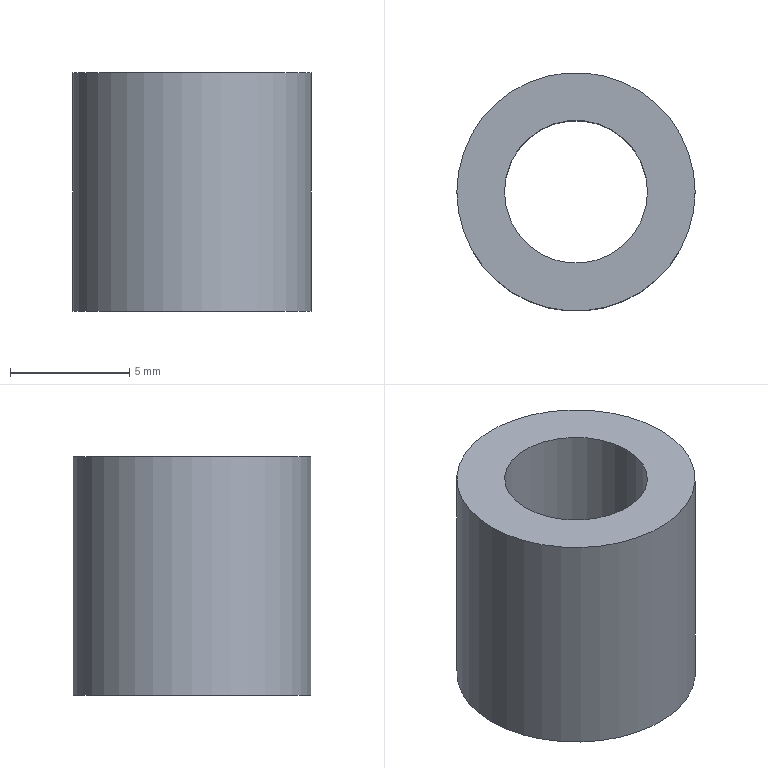Part | NX | features DATUM_CSYS 1, EXTRUDE 1 | 1 solid | 4 faces | box 10 x 10 x 10 mm | volume 502.655 mm3 | cylinder 2 | plane 2 | commonest cylinder face diameters 6 x1 10 x1
STEP:
#1=CARTESIAN_POINT('',(5.,0.,10.));
#2=VERTEX_POINT('',#1);
#3=CARTESIAN_POINT('',(0.,0.,10.));
#4=DIRECTION('',(0.,0.,1.));
#5=DIRECTION('',(1.,0.,0.));
#6=AXIS2_PLACEMENT_3D('',#3,#4,#5);
#7=CIRCLE('',#6,5.);
#8=EDGE_CURVE('',#2,#2,#7,.T.);
#9=ORIENTED_EDGE('',*,*,#8,.F.);
#10=EDGE_LOOP('',(#9));
#11=FACE_BOUND('',#10,.T.);
#12=CARTESIAN_POINT('',(5.,0.,0.));
#13=VERTEX_POINT('',#12);
#14=CARTESIAN_POINT('',(0.,0.,0.));
#15=DIRECTION('',(0.,0.,1.));
#16=DIRECTION('',(1.,0.,0.));
#17=AXIS2_PLACEMENT_3D('',#14,#15,#16);
#18=CIRCLE('',#17,5.);
#19=EDGE_CURVE('',#13,#13,#18,.T.);
#20=ORIENTED_EDGE('',*,*,#19,.T.);
#21=EDGE_LOOP('',(#20));
#22=FACE_BOUND('',#21,.T.);
#23=CARTESIAN_POINT('',(0.,0.,10.));
#24=DIRECTION('',(0.,0.,-1.));
#25=DIRECTION('',(-1.,0.,0.));
#26=AXIS2_PLACEMENT_3D('',#23,#24,#25);
#27=CYLINDRICAL_SURFACE('',#26,5.);
#28=ADVANCED_FACE('',(#11,#22),#27,.T.);
#29=CARTESIAN_POINT('',(3.,0.,10.));
#30=VERTEX_POINT('',#29);
#31=CARTESIAN_POINT('',(0.,0.,10.));
#32=DIRECTION('',(0.,0.,-1.));
#33=DIRECTION('',(1.,0.,0.));
#34=AXIS2_PLACEMENT_3D('',#31,#32,#33);
#35=CIRCLE('',#34,3.);
#36=EDGE_CURVE('',#30,#30,#35,.T.);
#37=ORIENTED_EDGE('',*,*,#36,.F.);
#38=EDGE_LOOP('',(#37));
#39=FACE_BOUND('',#38,.T.);
#40=CARTESIAN_POINT('',(3.,0.,0.));
#41=VERTEX_POINT('',#40);
#42=CARTESIAN_POINT('',(0.,0.,0.));
#43=DIRECTION('',(0.,0.,-1.));
#44=DIRECTION('',(1.,0.,0.));
#45=AXIS2_PLACEMENT_3D('',#42,#43,#44);
#46=CIRCLE('',#45,3.);
#47=EDGE_CURVE('',#41,#41,#46,.T.);
#48=ORIENTED_EDGE('',*,*,#47,.T.);
#49=EDGE_LOOP('',(#48));
#50=FACE_BOUND('',#49,.T.);
#51=CARTESIAN_POINT('',(0.,0.,10.));
#52=DIRECTION('',(0.,0.,-1.));
#53=DIRECTION('',(-1.,0.,0.));
#54=AXIS2_PLACEMENT_3D('',#51,#52,#53);
#55=CYLINDRICAL_SURFACE('',#54,3.);
#56=ADVANCED_FACE('',(#39,#50),#55,.F.);
#57=ORIENTED_EDGE('',*,*,#8,.T.);
#58=EDGE_LOOP('',(#57));
#59=FACE_BOUND('',#58,.T.);
#60=ORIENTED_EDGE('',*,*,#36,.T.);
#61=EDGE_LOOP('',(#60));
#62=FACE_BOUND('',#61,.T.);
#63=CARTESIAN_POINT('',(0.,0.,10.));
#64=DIRECTION('',(0.,0.,1.));
#65=DIRECTION('',(1.,0.,0.));
#66=AXIS2_PLACEMENT_3D('',#63,#64,#65);
#67=PLANE('',#66);
#68=ADVANCED_FACE('',(#59,#62),#67,.T.);
#69=ORIENTED_EDGE('',*,*,#19,.F.);
#70=EDGE_LOOP('',(#69));
#71=FACE_BOUND('',#70,.T.);
#72=ORIENTED_EDGE('',*,*,#47,.F.);
#73=EDGE_LOOP('',(#72));
#74=FACE_BOUND('',#73,.T.);
#75=CARTESIAN_POINT('',(0.,0.,0.));
#76=DIRECTION('',(0.,0.,1.));
#77=DIRECTION('',(1.,0.,0.));
#78=AXIS2_PLACEMENT_3D('',#75,#76,#77);
#79=PLANE('',#78);
#80=ADVANCED_FACE('',(#71,#74),#79,.F.);
#81=CLOSED_SHELL('',(#28,#56,#68,#80));
#82=MANIFOLD_SOLID_BREP('',#81);
#83=(LENGTH_UNIT()NAMED_UNIT(*)SI_UNIT(.MILLI.,.METRE.));
#84=UNCERTAINTY_MEASURE_WITH_UNIT(LENGTH_MEASURE(0.00001),#83,'','');
#85=(NAMED_UNIT(*)PLANE_ANGLE_UNIT()SI_UNIT($,.RADIAN.));
#86=(NAMED_UNIT(*)SI_UNIT($,.STERADIAN.)SOLID_ANGLE_UNIT());
#87=(GEOMETRIC_REPRESENTATION_CONTEXT(3)GLOBAL_UNCERTAINTY_ASSIGNED_CONTEXT((#84))GLOBAL_UNIT_ASSIGNED_CONTEXT((#83,#85,#86))REPRESENTATION_CONTEXT('',''));
#88=ADVANCED_BREP_SHAPE_REPRESENTATION('',(#82),#87);